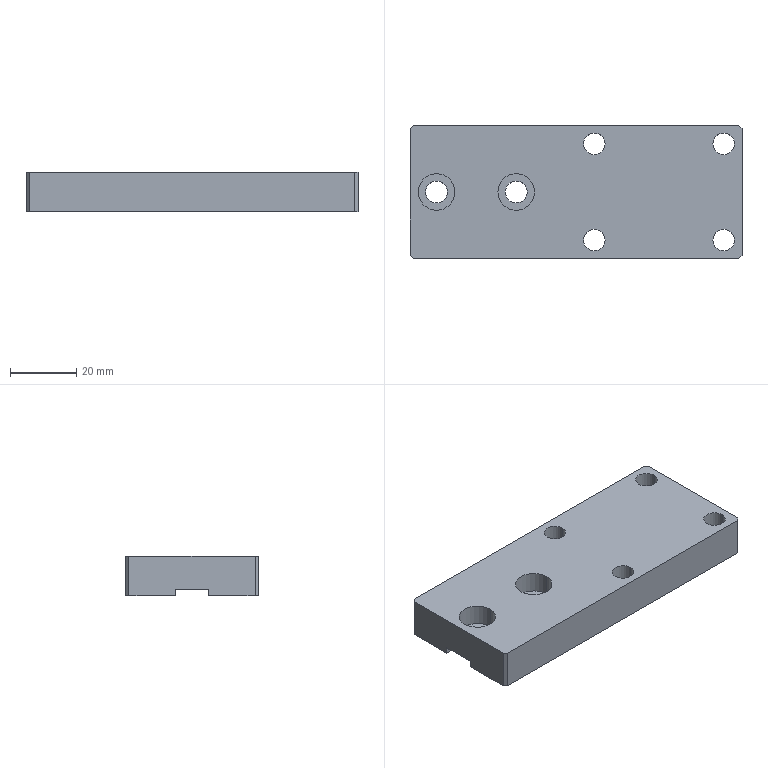Part | STEP file | 11-FG-B04711 | 1 solid | 32 faces | box 100 x 40 x 12 mm | volume 42920 mm3 | cylinder 16 | plane 16 | commonest cylinder face diameters 6.5 x8 6.6 x4 11 x4
STEP:
#1=CARTESIAN_POINT('',(-47.75,34.5,12.));
#2=VERTEX_POINT('',#1);
#3=CARTESIAN_POINT('',(-41.25,34.5,12.));
#4=VERTEX_POINT('',#3);
#5=CARTESIAN_POINT('',(-44.5,34.5,12.));
#6=DIRECTION('',(0.,0.,1.));
#7=DIRECTION('',(1.,0.,0.));
#8=AXIS2_PLACEMENT_3D('',#5,#6,#7);
#9=CIRCLE('',#8,3.25);
#10=EDGE_CURVE('',#2,#4,#9,.T.);
#11=ORIENTED_EDGE('',*,*,#10,.T.);
#12=CARTESIAN_POINT('',(-41.25,34.5,0.));
#13=VERTEX_POINT('',#12);
#14=CARTESIAN_POINT('',(-41.25,34.5,91.));
#15=DIRECTION('',(0.,0.,-1.));
#16=VECTOR('',#15,1000.);
#17=LINE('',#14,#16);
#18=EDGE_CURVE('',#4,#13,#17,.T.);
#19=ORIENTED_EDGE('',*,*,#18,.T.);
#20=CARTESIAN_POINT('',(-47.75,34.5,0.));
#21=VERTEX_POINT('',#20);
#22=CARTESIAN_POINT('',(-44.5,34.5,0.));
#23=DIRECTION('',(0.,0.,-1.));
#24=DIRECTION('',(-1.,0.,0.));
#25=AXIS2_PLACEMENT_3D('',#22,#23,#24);
#26=CIRCLE('',#25,3.25);
#27=EDGE_CURVE('',#13,#21,#26,.T.);
#28=ORIENTED_EDGE('',*,*,#27,.T.);
#29=CARTESIAN_POINT('',(-47.75,34.5,91.));
#30=DIRECTION('',(0.,0.,-1.));
#31=VECTOR('',#30,1000.);
#32=LINE('',#29,#31);
#33=EDGE_CURVE('',#2,#21,#32,.T.);
#34=ORIENTED_EDGE('',*,*,#33,.F.);
#35=EDGE_LOOP('',(#11,#19,#28,#34));
#36=FACE_OUTER_BOUND('',#35,.T.);
#37=CARTESIAN_POINT('',(-44.5,34.5,91.));
#38=DIRECTION('',(0.,0.,-1.));
#39=DIRECTION('',(-1.,0.,0.));
#40=AXIS2_PLACEMENT_3D('',#37,#38,#39);
#41=CYLINDRICAL_SURFACE('',#40,3.25);
#42=ADVANCED_FACE('',(#36),#41,.F.);
#43=CARTESIAN_POINT('',(-8.75,34.5,12.));
#44=VERTEX_POINT('',#43);
#45=CARTESIAN_POINT('',(-2.25,34.5,12.));
#46=VERTEX_POINT('',#45);
#47=CARTESIAN_POINT('',(-5.5,34.5,12.));
#48=DIRECTION('',(0.,0.,1.));
#49=DIRECTION('',(1.,0.,0.));
#50=AXIS2_PLACEMENT_3D('',#47,#48,#49);
#51=CIRCLE('',#50,3.25);
#52=EDGE_CURVE('',#44,#46,#51,.T.);
#53=ORIENTED_EDGE('',*,*,#52,.T.);
#54=CARTESIAN_POINT('',(-2.25,34.5,0.));
#55=VERTEX_POINT('',#54);
#56=CARTESIAN_POINT('',(-2.25,34.5,91.));
#57=DIRECTION('',(0.,0.,-1.));
#58=VECTOR('',#57,1000.);
#59=LINE('',#56,#58);
#60=EDGE_CURVE('',#46,#55,#59,.T.);
#61=ORIENTED_EDGE('',*,*,#60,.T.);
#62=CARTESIAN_POINT('',(-8.75,34.5,0.));
#63=VERTEX_POINT('',#62);
#64=CARTESIAN_POINT('',(-5.5,34.5,0.));
#65=DIRECTION('',(0.,0.,-1.));
#66=DIRECTION('',(-1.,0.,0.));
#67=AXIS2_PLACEMENT_3D('',#64,#65,#66);
#68=CIRCLE('',#67,3.25);
#69=EDGE_CURVE('',#55,#63,#68,.T.);
#70=ORIENTED_EDGE('',*,*,#69,.T.);
#71=CARTESIAN_POINT('',(-8.75,34.5,91.));
#72=DIRECTION('',(0.,0.,-1.));
#73=VECTOR('',#72,1000.);
#74=LINE('',#71,#73);
#75=EDGE_CURVE('',#44,#63,#74,.T.);
#76=ORIENTED_EDGE('',*,*,#75,.F.);
#77=EDGE_LOOP('',(#53,#61,#70,#76));
#78=FACE_OUTER_BOUND('',#77,.T.);
#79=CARTESIAN_POINT('',(-5.5,34.5,91.));
#80=DIRECTION('',(0.,0.,-1.));
#81=DIRECTION('',(-1.,0.,0.));
#82=AXIS2_PLACEMENT_3D('',#79,#80,#81);
#83=CYLINDRICAL_SURFACE('',#82,3.25);
#84=ADVANCED_FACE('',(#78),#83,.F.);
#85=CARTESIAN_POINT('',(-8.75,5.5,12.));
#86=VERTEX_POINT('',#85);
#87=CARTESIAN_POINT('',(-2.25,5.5,12.));
#88=VERTEX_POINT('',#87);
#89=CARTESIAN_POINT('',(-5.5,5.5,12.));
#90=DIRECTION('',(0.,0.,1.));
#91=DIRECTION('',(1.,0.,0.));
#92=AXIS2_PLACEMENT_3D('',#89,#90,#91);
#93=CIRCLE('',#92,3.25);
#94=EDGE_CURVE('',#86,#88,#93,.T.);
#95=ORIENTED_EDGE('',*,*,#94,.T.);
#96=CARTESIAN_POINT('',(-2.25,5.5,0.));
#97=VERTEX_POINT('',#96);
#98=CARTESIAN_POINT('',(-2.25,5.5,91.));
#99=DIRECTION('',(0.,0.,-1.));
#100=VECTOR('',#99,1000.);
#101=LINE('',#98,#100);
#102=EDGE_CURVE('',#88,#97,#101,.T.);
#103=ORIENTED_EDGE('',*,*,#102,.T.);
#104=CARTESIAN_POINT('',(-8.75,5.5,0.));
#105=VERTEX_POINT('',#104);
#106=CARTESIAN_POINT('',(-5.5,5.5,0.));
#107=DIRECTION('',(0.,0.,-1.));
#108=DIRECTION('',(-1.,0.,0.));
#109=AXIS2_PLACEMENT_3D('',#106,#107,#108);
#110=CIRCLE('',#109,3.25);
#111=EDGE_CURVE('',#97,#105,#110,.T.);
#112=ORIENTED_EDGE('',*,*,#111,.T.);
#113=CARTESIAN_POINT('',(-8.75,5.5,91.));
#114=DIRECTION('',(0.,0.,-1.));
#115=VECTOR('',#114,1000.);
#116=LINE('',#113,#115);
#117=EDGE_CURVE('',#86,#105,#116,.T.);
#118=ORIENTED_EDGE('',*,*,#117,.F.);
#119=EDGE_LOOP('',(#95,#103,#112,#118));
#120=FACE_OUTER_BOUND('',#119,.T.);
#121=CARTESIAN_POINT('',(-5.5,5.5,91.));
#122=DIRECTION('',(0.,0.,-1.));
#123=DIRECTION('',(-1.,0.,0.));
#124=AXIS2_PLACEMENT_3D('',#121,#122,#123);
#125=CYLINDRICAL_SURFACE('',#124,3.25);
#126=ADVANCED_FACE('',(#120),#125,.F.);
#127=CARTESIAN_POINT('',(-47.75,5.5,12.));
#128=VERTEX_POINT('',#127);
#129=CARTESIAN_POINT('',(-41.25,5.5,12.));
#130=VERTEX_POINT('',#129);
#131=CARTESIAN_POINT('',(-44.5,5.5,12.));
#132=DIRECTION('',(0.,0.,1.));
#133=DIRECTION('',(1.,0.,0.));
#134=AXIS2_PLACEMENT_3D('',#131,#132,#133);
#135=CIRCLE('',#134,3.25);
#136=EDGE_CURVE('',#128,#130,#135,.T.);
#137=ORIENTED_EDGE('',*,*,#136,.T.);
#138=CARTESIAN_POINT('',(-41.25,5.5,0.));
#139=VERTEX_POINT('',#138);
#140=CARTESIAN_POINT('',(-41.25,5.5,91.));
#141=DIRECTION('',(0.,0.,-1.));
#142=VECTOR('',#141,1000.);
#143=LINE('',#140,#142);
#144=EDGE_CURVE('',#130,#139,#143,.T.);
#145=ORIENTED_EDGE('',*,*,#144,.T.);
#146=CARTESIAN_POINT('',(-47.75,5.5,0.));
#147=VERTEX_POINT('',#146);
#148=CARTESIAN_POINT('',(-44.5,5.5,0.));
#149=DIRECTION('',(0.,0.,-1.));
#150=DIRECTION('',(-1.,0.,0.));
#151=AXIS2_PLACEMENT_3D('',#148,#149,#150);
#152=CIRCLE('',#151,3.25);
#153=EDGE_CURVE('',#139,#147,#152,.T.);
#154=ORIENTED_EDGE('',*,*,#153,.T.);
#155=CARTESIAN_POINT('',(-47.75,5.5,91.));
#156=DIRECTION('',(0.,0.,-1.));
#157=VECTOR('',#156,1000.);
#158=LINE('',#155,#157);
#159=EDGE_CURVE('',#128,#147,#158,.T.);
#160=ORIENTED_EDGE('',*,*,#159,.F.);
#161=EDGE_LOOP('',(#137,#145,#154,#160));
#162=FACE_OUTER_BOUND('',#161,.T.);
#163=CARTESIAN_POINT('',(-44.5,5.5,91.));
#164=DIRECTION('',(0.,0.,-1.));
#165=DIRECTION('',(-1.,0.,0.));
#166=AXIS2_PLACEMENT_3D('',#163,#164,#165);
#167=CYLINDRICAL_SURFACE('',#166,3.25);
#168=ADVANCED_FACE('',(#162),#167,.F.);
#169=CARTESIAN_POINT('',(-97.5,20.,5.6));
#170=VERTEX_POINT('',#169);
#171=CARTESIAN_POINT('',(-86.5,20.,5.6));
#172=VERTEX_POINT('',#171);
#173=CARTESIAN_POINT('',(-92.,20.,5.6));
#174=DIRECTION('',(0.,0.,1.));
#175=DIRECTION('',(1.,0.,0.));
#176=AXIS2_PLACEMENT_3D('',#173,#174,#175);
#177=CIRCLE('',#176,5.5);
#178=EDGE_CURVE('',#170,#172,#177,.T.);
#179=ORIENTED_EDGE('',*,*,#178,.F.);
#180=CARTESIAN_POINT('',(-97.5,20.,12.));
#181=VERTEX_POINT('',#180);
#182=CARTESIAN_POINT('',(-97.5,20.,12.));
#183=DIRECTION('',(0.,0.,1.));
#184=VECTOR('',#183,1000.);
#185=LINE('',#182,#184);
#186=EDGE_CURVE('',#170,#181,#185,.T.);
#187=ORIENTED_EDGE('',*,*,#186,.T.);
#188=CARTESIAN_POINT('',(-86.5,20.,12.));
#189=VERTEX_POINT('',#188);
#190=CARTESIAN_POINT('',(-92.,20.,12.));
#191=DIRECTION('',(0.,0.,1.));
#192=DIRECTION('',(1.,0.,0.));
#193=AXIS2_PLACEMENT_3D('',#190,#191,#192);
#194=CIRCLE('',#193,5.5);
#195=EDGE_CURVE('',#181,#189,#194,.T.);
#196=ORIENTED_EDGE('',*,*,#195,.T.);
#197=CARTESIAN_POINT('',(-86.5,20.,12.));
#198=DIRECTION('',(0.,0.,1.));
#199=VECTOR('',#198,1000.);
#200=LINE('',#197,#199);
#201=EDGE_CURVE('',#172,#189,#200,.T.);
#202=ORIENTED_EDGE('',*,*,#201,.F.);
#203=EDGE_LOOP('',(#179,#187,#196,#202));
#204=FACE_OUTER_BOUND('',#203,.T.);
#205=CARTESIAN_POINT('',(-92.,20.,12.));
#206=DIRECTION('',(0.,0.,1.));
#207=DIRECTION('',(1.,0.,0.));
#208=AXIS2_PLACEMENT_3D('',#205,#206,#207);
#209=CYLINDRICAL_SURFACE('',#208,5.5);
#210=ADVANCED_FACE('',(#204),#209,.F.);
#211=CARTESIAN_POINT('',(-95.3,20.,2.));
#212=VERTEX_POINT('',#211);
#213=CARTESIAN_POINT('',(-88.7,20.,2.));
#214=VERTEX_POINT('',#213);
#215=CARTESIAN_POINT('',(-92.,20.,2.));
#216=DIRECTION('',(0.,0.,1.));
#217=DIRECTION('',(1.,0.,0.));
#218=AXIS2_PLACEMENT_3D('',#215,#216,#217);
#219=CIRCLE('',#218,3.3);
#220=EDGE_CURVE('',#212,#214,#219,.T.);
#221=ORIENTED_EDGE('',*,*,#220,.F.);
#222=CARTESIAN_POINT('',(-95.3,20.,5.6));
#223=VERTEX_POINT('',#222);
#224=CARTESIAN_POINT('',(-95.3,20.,12.));
#225=DIRECTION('',(0.,0.,1.));
#226=VECTOR('',#225,1000.);
#227=LINE('',#224,#226);
#228=EDGE_CURVE('',#212,#223,#227,.T.);
#229=ORIENTED_EDGE('',*,*,#228,.T.);
#230=CARTESIAN_POINT('',(-88.7,20.,5.6));
#231=VERTEX_POINT('',#230);
#232=CARTESIAN_POINT('',(-92.,20.,5.6));
#233=DIRECTION('',(0.,0.,1.));
#234=DIRECTION('',(1.,0.,0.));
#235=AXIS2_PLACEMENT_3D('',#232,#233,#234);
#236=CIRCLE('',#235,3.3);
#237=EDGE_CURVE('',#223,#231,#236,.T.);
#238=ORIENTED_EDGE('',*,*,#237,.T.);
#239=CARTESIAN_POINT('',(-88.7,20.,12.));
#240=DIRECTION('',(0.,0.,1.));
#241=VECTOR('',#240,1000.);
#242=LINE('',#239,#241);
#243=EDGE_CURVE('',#214,#231,#242,.T.);
#244=ORIENTED_EDGE('',*,*,#243,.F.);
#245=EDGE_LOOP('',(#221,#229,#238,#244));
#246=FACE_OUTER_BOUND('',#245,.T.);
#247=CARTESIAN_POINT('',(-92.,20.,12.));
#248=DIRECTION('',(0.,0.,1.));
#249=DIRECTION('',(1.,0.,0.));
#250=AXIS2_PLACEMENT_3D('',#247,#248,#249);
#251=CYLINDRICAL_SURFACE('',#250,3.3);
#252=ADVANCED_FACE('',(#246),#251,.F.);
#253=CARTESIAN_POINT('',(-73.5,20.,5.6));
#254=VERTEX_POINT('',#253);
#255=CARTESIAN_POINT('',(-62.5,20.,5.6));
#256=VERTEX_POINT('',#255);
#257=CARTESIAN_POINT('',(-68.,20.,5.6));
#258=DIRECTION('',(0.,0.,1.));
#259=DIRECTION('',(1.,0.,0.));
#260=AXIS2_PLACEMENT_3D('',#257,#258,#259);
#261=CIRCLE('',#260,5.5);
#262=EDGE_CURVE('',#254,#256,#261,.T.);
#263=ORIENTED_EDGE('',*,*,#262,.F.);
#264=CARTESIAN_POINT('',(-73.5,20.,12.));
#265=VERTEX_POINT('',#264);
#266=CARTESIAN_POINT('',(-73.5,20.,12.));
#267=DIRECTION('',(0.,0.,1.));
#268=VECTOR('',#267,1000.);
#269=LINE('',#266,#268);
#270=EDGE_CURVE('',#254,#265,#269,.T.);
#271=ORIENTED_EDGE('',*,*,#270,.T.);
#272=CARTESIAN_POINT('',(-62.5,20.,12.));
#273=VERTEX_POINT('',#272);
#274=CARTESIAN_POINT('',(-68.,20.,12.));
#275=DIRECTION('',(0.,0.,1.));
#276=DIRECTION('',(1.,0.,0.));
#277=AXIS2_PLACEMENT_3D('',#274,#275,#276);
#278=CIRCLE('',#277,5.5);
#279=EDGE_CURVE('',#265,#273,#278,.T.);
#280=ORIENTED_EDGE('',*,*,#279,.T.);
#281=CARTESIAN_POINT('',(-62.5,20.,12.));
#282=DIRECTION('',(0.,0.,1.));
#283=VECTOR('',#282,1000.);
#284=LINE('',#281,#283);
#285=EDGE_CURVE('',#256,#273,#284,.T.);
#286=ORIENTED_EDGE('',*,*,#285,.F.);
#287=EDGE_LOOP('',(#263,#271,#280,#286));
#288=FACE_OUTER_BOUND('',#287,.T.);
#289=CARTESIAN_POINT('',(-68.,20.,12.));
#290=DIRECTION('',(0.,0.,1.));
#291=DIRECTION('',(1.,0.,0.));
#292=AXIS2_PLACEMENT_3D('',#289,#290,#291);
#293=CYLINDRICAL_SURFACE('',#292,5.5);
#294=ADVANCED_FACE('',(#288),#293,.F.);
#295=CARTESIAN_POINT('',(-71.3,20.,2.));
#296=VERTEX_POINT('',#295);
#297=CARTESIAN_POINT('',(-64.7,20.,2.));
#298=VERTEX_POINT('',#297);
#299=CARTESIAN_POINT('',(-68.,20.,2.));
#300=DIRECTION('',(0.,0.,1.));
#301=DIRECTION('',(1.,0.,0.));
#302=AXIS2_PLACEMENT_3D('',#299,#300,#301);
#303=CIRCLE('',#302,3.3);
#304=EDGE_CURVE('',#296,#298,#303,.T.);
#305=ORIENTED_EDGE('',*,*,#304,.F.);
#306=CARTESIAN_POINT('',(-71.3,20.,5.6));
#307=VERTEX_POINT('',#306);
#308=CARTESIAN_POINT('',(-71.3,20.,12.));
#309=DIRECTION('',(0.,0.,1.));
#310=VECTOR('',#309,1000.);
#311=LINE('',#308,#310);
#312=EDGE_CURVE('',#296,#307,#311,.T.);
#313=ORIENTED_EDGE('',*,*,#312,.T.);
#314=CARTESIAN_POINT('',(-64.7,20.,5.6));
#315=VERTEX_POINT('',#314);
#316=CARTESIAN_POINT('',(-68.,20.,5.6));
#317=DIRECTION('',(0.,0.,1.));
#318=DIRECTION('',(1.,0.,0.));
#319=AXIS2_PLACEMENT_3D('',#316,#317,#318);
#320=CIRCLE('',#319,3.3);
#321=EDGE_CURVE('',#307,#315,#320,.T.);
#322=ORIENTED_EDGE('',*,*,#321,.T.);
#323=CARTESIAN_POINT('',(-64.7,20.,12.));
#324=DIRECTION('',(0.,0.,1.));
#325=VECTOR('',#324,1000.);
#326=LINE('',#323,#325);
#327=EDGE_CURVE('',#298,#315,#326,.T.);
#328=ORIENTED_EDGE('',*,*,#327,.F.);
#329=EDGE_LOOP('',(#305,#313,#322,#328));
#330=FACE_OUTER_BOUND('',#329,.T.);
#331=CARTESIAN_POINT('',(-68.,20.,12.));
#332=DIRECTION('',(0.,0.,1.));
#333=DIRECTION('',(1.,0.,0.));
#334=AXIS2_PLACEMENT_3D('',#331,#332,#333);
#335=CYLINDRICAL_SURFACE('',#334,3.3);
#336=ADVANCED_FACE('',(#330),#335,.F.);
#337=CARTESIAN_POINT('',(-44.5,34.5,0.));
#338=DIRECTION('',(0.,0.,-1.));
#339=DIRECTION('',(-1.,0.,0.));
#340=AXIS2_PLACEMENT_3D('',#337,#338,#339);
#341=CIRCLE('',#340,3.25);
#342=EDGE_CURVE('',#21,#13,#341,.T.);
#343=ORIENTED_EDGE('',*,*,#342,.F.);
#344=ORIENTED_EDGE('',*,*,#27,.F.);
#345=EDGE_LOOP('',(#343,#344));
#346=FACE_BOUND('',#345,.T.);
#347=CARTESIAN_POINT('',(-5.5,34.5,0.));
#348=DIRECTION('',(0.,0.,-1.));
#349=DIRECTION('',(-1.,0.,0.));
#350=AXIS2_PLACEMENT_3D('',#347,#348,#349);
#351=CIRCLE('',#350,3.25);
#352=EDGE_CURVE('',#63,#55,#351,.T.);
#353=ORIENTED_EDGE('',*,*,#352,.F.);
#354=ORIENTED_EDGE('',*,*,#69,.F.);
#355=EDGE_LOOP('',(#353,#354));
#356=FACE_BOUND('',#355,.T.);
#357=CARTESIAN_POINT('',(0.,25.,0.));
#358=VERTEX_POINT('',#357);
#359=CARTESIAN_POINT('',(0.,39.,0.));
#360=VERTEX_POINT('',#359);
#361=CARTESIAN_POINT('',(0.,40.,0.));
#362=DIRECTION('',(0.,1.,0.));
#363=VECTOR('',#362,1000.);
#364=LINE('',#361,#363);
#365=EDGE_CURVE('',#358,#360,#364,.T.);
#366=ORIENTED_EDGE('',*,*,#365,.F.);
#367=CARTESIAN_POINT('',(-100.,25.,0.));
#368=VERTEX_POINT('',#367);
#369=CARTESIAN_POINT('',(-100.,25.,0.));
#370=DIRECTION('',(-1.,0.,0.));
#371=VECTOR('',#370,1000.);
#372=LINE('',#369,#371);
#373=EDGE_CURVE('',#358,#368,#372,.T.);
#374=ORIENTED_EDGE('',*,*,#373,.T.);
#375=CARTESIAN_POINT('',(-100.,39.,0.));
#376=VERTEX_POINT('',#375);
#377=CARTESIAN_POINT('',(-100.,40.,0.));
#378=DIRECTION('',(0.,-1.,0.));
#379=VECTOR('',#378,1000.);
#380=LINE('',#377,#379);
#381=EDGE_CURVE('',#376,#368,#380,.T.);
#382=ORIENTED_EDGE('',*,*,#381,.F.);
#383=CARTESIAN_POINT('',(-99.,40.,0.));
#384=VERTEX_POINT('',#383);
#385=CARTESIAN_POINT('',(-100.,39.,0.));
#386=DIRECTION('',(0.7071,0.7071,0.));
#387=VECTOR('',#386,1000.);
#388=LINE('',#385,#387);
#389=EDGE_CURVE('',#376,#384,#388,.T.);
#390=ORIENTED_EDGE('',*,*,#389,.T.);
#391=CARTESIAN_POINT('',(-1.,40.,0.));
#392=VERTEX_POINT('',#391);
#393=CARTESIAN_POINT('',(-100.,40.,0.));
#394=DIRECTION('',(-1.,0.,0.));
#395=VECTOR('',#394,1000.);
#396=LINE('',#393,#395);
#397=EDGE_CURVE('',#392,#384,#396,.T.);
#398=ORIENTED_EDGE('',*,*,#397,.F.);
#399=CARTESIAN_POINT('',(-1.,40.,0.));
#400=DIRECTION('',(0.7071,-0.7071,0.));
#401=VECTOR('',#400,1000.);
#402=LINE('',#399,#401);
#403=EDGE_CURVE('',#392,#360,#402,.T.);
#404=ORIENTED_EDGE('',*,*,#403,.T.);
#405=EDGE_LOOP('',(#366,#374,#382,#390,#398,#404));
#406=FACE_OUTER_BOUND('',#405,.T.);
#407=CARTESIAN_POINT('',(-100.,0.,0.));
#408=DIRECTION('',(0.,0.,1.));
#409=DIRECTION('',(1.,0.,0.));
#410=AXIS2_PLACEMENT_3D('',#407,#408,#409);
#411=PLANE('',#410);
#412=ADVANCED_FACE('',(#346,#356,#406),#411,.F.);
#413=ORIENTED_EDGE('',*,*,#381,.T.);
#414=CARTESIAN_POINT('',(-100.,25.,2.));
#415=VERTEX_POINT('',#414);
#416=CARTESIAN_POINT('',(-100.,25.,0.));
#417=DIRECTION('',(0.,0.,-1.));
#418=VECTOR('',#417,1000.);
#419=LINE('',#416,#418);
#420=EDGE_CURVE('',#415,#368,#419,.T.);
#421=ORIENTED_EDGE('',*,*,#420,.F.);
#422=CARTESIAN_POINT('',(-100.,15.,2.));
#423=VERTEX_POINT('',#422);
#424=CARTESIAN_POINT('',(-100.,15.,2.));
#425=DIRECTION('',(0.,1.,0.));
#426=VECTOR('',#425,1000.);
#427=LINE('',#424,#426);
#428=EDGE_CURVE('',#423,#415,#427,.T.);
#429=ORIENTED_EDGE('',*,*,#428,.F.);
#430=CARTESIAN_POINT('',(-100.,15.,0.));
#431=VERTEX_POINT('',#430);
#432=CARTESIAN_POINT('',(-100.,15.,0.));
#433=DIRECTION('',(0.,0.,1.));
#434=VECTOR('',#433,1000.);
#435=LINE('',#432,#434);
#436=EDGE_CURVE('',#431,#423,#435,.T.);
#437=ORIENTED_EDGE('',*,*,#436,.F.);
#438=CARTESIAN_POINT('',(-100.,1.,0.));
#439=VERTEX_POINT('',#438);
#440=CARTESIAN_POINT('',(-100.,40.,0.));
#441=DIRECTION('',(0.,-1.,0.));
#442=VECTOR('',#441,1000.);
#443=LINE('',#440,#442);
#444=EDGE_CURVE('',#431,#439,#443,.T.);
#445=ORIENTED_EDGE('',*,*,#444,.T.);
#446=CARTESIAN_POINT('',(-100.,1.,12.));
#447=VERTEX_POINT('',#446);
#448=CARTESIAN_POINT('',(-100.,1.,12.));
#449=DIRECTION('',(0.,0.,1.));
#450=VECTOR('',#449,1000.);
#451=LINE('',#448,#450);
#452=EDGE_CURVE('',#439,#447,#451,.T.);
#453=ORIENTED_EDGE('',*,*,#452,.T.);
#454=CARTESIAN_POINT('',(-100.,39.,12.));
#455=VERTEX_POINT('',#454);
#456=CARTESIAN_POINT('',(-100.,40.,12.));
#457=DIRECTION('',(0.,-1.,0.));
#458=VECTOR('',#457,1000.);
#459=LINE('',#456,#458);
#460=EDGE_CURVE('',#455,#447,#459,.T.);
#461=ORIENTED_EDGE('',*,*,#460,.F.);
#462=CARTESIAN_POINT('',(-100.,39.,12.));
#463=DIRECTION('',(0.,0.,-1.));
#464=VECTOR('',#463,1000.);
#465=LINE('',#462,#464);
#466=EDGE_CURVE('',#455,#376,#465,.T.);
#467=ORIENTED_EDGE('',*,*,#466,.T.);
#468=EDGE_LOOP('',(#413,#421,#429,#437,#445,#453,#461,#467));
#469=FACE_OUTER_BOUND('',#468,.T.);
#470=CARTESIAN_POINT('',(-100.,40.,12.));
#471=DIRECTION('',(1.,0.,0.));
#472=DIRECTION('',(0.,0.,-1.));
#473=AXIS2_PLACEMENT_3D('',#470,#471,#472);
#474=PLANE('',#473);
#475=ADVANCED_FACE('',(#469),#474,.F.);
#476=CARTESIAN_POINT('',(-99.,0.,12.));
#477=VERTEX_POINT('',#476);
#478=CARTESIAN_POINT('',(-1.,0.,12.));
#479=VERTEX_POINT('',#478);
#480=CARTESIAN_POINT('',(-100.,0.,12.));
#481=DIRECTION('',(1.,0.,0.));
#482=VECTOR('',#481,1000.);
#483=LINE('',#480,#482);
#484=EDGE_CURVE('',#477,#479,#483,.T.);
#485=ORIENTED_EDGE('',*,*,#484,.F.);
#486=CARTESIAN_POINT('',(-99.,0.,0.));
#487=VERTEX_POINT('',#486);
#488=CARTESIAN_POINT('',(-99.,0.,12.));
#489=DIRECTION('',(0.,0.,-1.));
#490=VECTOR('',#489,1000.);
#491=LINE('',#488,#490);
#492=EDGE_CURVE('',#477,#487,#491,.T.);
#493=ORIENTED_EDGE('',*,*,#492,.T.);
#494=CARTESIAN_POINT('',(-1.,0.,0.));
#495=VERTEX_POINT('',#494);
#496=CARTESIAN_POINT('',(-100.,0.,0.));
#497=DIRECTION('',(1.,0.,0.));
#498=VECTOR('',#497,1000.);
#499=LINE('',#496,#498);
#500=EDGE_CURVE('',#487,#495,#499,.T.);
#501=ORIENTED_EDGE('',*,*,#500,.T.);
#502=CARTESIAN_POINT('',(-1.,0.,12.));
#503=DIRECTION('',(0.,0.,1.));
#504=VECTOR('',#503,1000.);
#505=LINE('',#502,#504);
#506=EDGE_CURVE('',#495,#479,#505,.T.);
#507=ORIENTED_EDGE('',*,*,#506,.T.);
#508=EDGE_LOOP('',(#485,#493,#501,#507));
#509=FACE_OUTER_BOUND('',#508,.T.);
#510=CARTESIAN_POINT('',(-100.,0.,12.));
#511=DIRECTION('',(0.,1.,0.));
#512=DIRECTION('',(0.,0.,1.));
#513=AXIS2_PLACEMENT_3D('',#510,#511,#512);
#514=PLANE('',#513);
#515=ADVANCED_FACE('',(#509),#514,.F.);
#516=CARTESIAN_POINT('',(0.,15.,2.));
#517=VERTEX_POINT('',#516);
#518=CARTESIAN_POINT('',(0.,25.,2.));
#519=VERTEX_POINT('',#518);
#520=CARTESIAN_POINT('',(0.,40.,2.));
#521=DIRECTION('',(0.,1.,0.));
#522=VECTOR('',#521,1000.);
#523=LINE('',#520,#522);
#524=EDGE_CURVE('',#517,#519,#523,.T.);
#525=ORIENTED_EDGE('',*,*,#524,.T.);
#526=CARTESIAN_POINT('',(0.,25.,12.));
#527=DIRECTION('',(0.,0.,-1.));
#528=VECTOR('',#527,1000.);
#529=LINE('',#526,#528);
#530=EDGE_CURVE('',#519,#358,#529,.T.);
#531=ORIENTED_EDGE('',*,*,#530,.T.);
#532=ORIENTED_EDGE('',*,*,#365,.T.);
#533=CARTESIAN_POINT('',(0.,39.,12.));
#534=VERTEX_POINT('',#533);
#535=CARTESIAN_POINT('',(0.,39.,12.));
#536=DIRECTION('',(0.,0.,1.));
#537=VECTOR('',#536,1000.);
#538=LINE('',#535,#537);
#539=EDGE_CURVE('',#360,#534,#538,.T.);
#540=ORIENTED_EDGE('',*,*,#539,.T.);
#541=CARTESIAN_POINT('',(0.,1.,12.));
#542=VERTEX_POINT('',#541);
#543=CARTESIAN_POINT('',(0.,40.,12.));
#544=DIRECTION('',(0.,1.,0.));
#545=VECTOR('',#544,1000.);
#546=LINE('',#543,#545);
#547=EDGE_CURVE('',#542,#534,#546,.T.);
#548=ORIENTED_EDGE('',*,*,#547,.F.);
#549=CARTESIAN_POINT('',(0.,1.,0.));
#550=VERTEX_POINT('',#549);
#551=CARTESIAN_POINT('',(0.,1.,12.));
#552=DIRECTION('',(0.,0.,-1.));
#553=VECTOR('',#552,1000.);
#554=LINE('',#551,#553);
#555=EDGE_CURVE('',#542,#550,#554,.T.);
#556=ORIENTED_EDGE('',*,*,#555,.T.);
#557=CARTESIAN_POINT('',(0.,15.,0.));
#558=VERTEX_POINT('',#557);
#559=CARTESIAN_POINT('',(0.,40.,0.));
#560=DIRECTION('',(0.,1.,0.));
#561=VECTOR('',#560,1000.);
#562=LINE('',#559,#561);
#563=EDGE_CURVE('',#550,#558,#562,.T.);
#564=ORIENTED_EDGE('',*,*,#563,.T.);
#565=CARTESIAN_POINT('',(0.,15.,12.));
#566=DIRECTION('',(0.,0.,1.));
#567=VECTOR('',#566,1000.);
#568=LINE('',#565,#567);
#569=EDGE_CURVE('',#558,#517,#568,.T.);
#570=ORIENTED_EDGE('',*,*,#569,.T.);
#571=EDGE_LOOP('',(#525,#531,#532,#540,#548,#556,#564,#570));
#572=FACE_OUTER_BOUND('',#571,.T.);
#573=CARTESIAN_POINT('',(0.,40.,12.));
#574=DIRECTION('',(-1.,0.,0.));
#575=DIRECTION('',(0.,-1.,0.));
#576=AXIS2_PLACEMENT_3D('',#573,#574,#575);
#577=PLANE('',#576);
#578=ADVANCED_FACE('',(#572),#577,.F.);
#579=CARTESIAN_POINT('',(-1.,40.,12.));
#580=VERTEX_POINT('',#579);
#581=CARTESIAN_POINT('',(-99.,40.,12.));
#582=VERTEX_POINT('',#581);
#583=CARTESIAN_POINT('',(-100.,40.,12.));
#584=DIRECTION('',(-1.,0.,0.));
#585=VECTOR('',#584,1000.);
#586=LINE('',#583,#585);
#587=EDGE_CURVE('',#580,#582,#586,.T.);
#588=ORIENTED_EDGE('',*,*,#587,.F.);
#589=CARTESIAN_POINT('',(-1.,40.,12.));
#590=DIRECTION('',(0.,0.,-1.));
#591=VECTOR('',#590,1000.);
#592=LINE('',#589,#591);
#593=EDGE_CURVE('',#580,#392,#592,.T.);
#594=ORIENTED_EDGE('',*,*,#593,.T.);
#595=ORIENTED_EDGE('',*,*,#397,.T.);
#596=CARTESIAN_POINT('',(-99.,40.,12.));
#597=DIRECTION('',(0.,0.,1.));
#598=VECTOR('',#597,1000.);
#599=LINE('',#596,#598);
#600=EDGE_CURVE('',#384,#582,#599,.T.);
#601=ORIENTED_EDGE('',*,*,#600,.T.);
#602=EDGE_LOOP('',(#588,#594,#595,#601));
#603=FACE_OUTER_BOUND('',#602,.T.);
#604=CARTESIAN_POINT('',(-100.,40.,12.));
#605=DIRECTION('',(0.,-1.,0.));
#606=DIRECTION('',(0.,0.,-1.));
#607=AXIS2_PLACEMENT_3D('',#604,#605,#606);
#608=PLANE('',#607);
#609=ADVANCED_FACE('',(#603),#608,.F.);
#610=ORIENTED_EDGE('',*,*,#94,.F.);
#611=CARTESIAN_POINT('',(-5.5,5.5,12.));
#612=DIRECTION('',(0.,0.,1.));
#613=DIRECTION('',(1.,0.,0.));
#614=AXIS2_PLACEMENT_3D('',#611,#612,#613);
#615=CIRCLE('',#614,3.25);
#616=EDGE_CURVE('',#88,#86,#615,.T.);
#617=ORIENTED_EDGE('',*,*,#616,.F.);
#618=EDGE_LOOP('',(#610,#617));
#619=FACE_BOUND('',#618,.T.);
#620=ORIENTED_EDGE('',*,*,#10,.F.);
#621=CARTESIAN_POINT('',(-44.5,34.5,12.));
#622=DIRECTION('',(0.,0.,1.));
#623=DIRECTION('',(1.,0.,0.));
#624=AXIS2_PLACEMENT_3D('',#621,#622,#623);
#625=CIRCLE('',#624,3.25);
#626=EDGE_CURVE('',#4,#2,#625,.T.);
#627=ORIENTED_EDGE('',*,*,#626,.F.);
#628=EDGE_LOOP('',(#620,#627));
#629=FACE_BOUND('',#628,.T.);
#630=ORIENTED_EDGE('',*,*,#52,.F.);
#631=CARTESIAN_POINT('',(-5.5,34.5,12.));
#632=DIRECTION('',(0.,0.,1.));
#633=DIRECTION('',(1.,0.,0.));
#634=AXIS2_PLACEMENT_3D('',#631,#632,#633);
#635=CIRCLE('',#634,3.25);
#636=EDGE_CURVE('',#46,#44,#635,.T.);
#637=ORIENTED_EDGE('',*,*,#636,.F.);
#638=EDGE_LOOP('',(#630,#637));
#639=FACE_BOUND('',#638,.T.);
#640=ORIENTED_EDGE('',*,*,#136,.F.);
#641=CARTESIAN_POINT('',(-44.5,5.5,12.));
#642=DIRECTION('',(0.,0.,1.));
#643=DIRECTION('',(1.,0.,0.));
#644=AXIS2_PLACEMENT_3D('',#641,#642,#643);
#645=CIRCLE('',#644,3.25);
#646=EDGE_CURVE('',#130,#128,#645,.T.);
#647=ORIENTED_EDGE('',*,*,#646,.F.);
#648=EDGE_LOOP('',(#640,#647));
#649=FACE_BOUND('',#648,.T.);
#650=CARTESIAN_POINT('',(-92.,20.,12.));
#651=DIRECTION('',(0.,0.,1.));
#652=DIRECTION('',(1.,0.,0.));
#653=AXIS2_PLACEMENT_3D('',#650,#651,#652);
#654=CIRCLE('',#653,5.5);
#655=EDGE_CURVE('',#189,#181,#654,.T.);
#656=ORIENTED_EDGE('',*,*,#655,.F.);
#657=ORIENTED_EDGE('',*,*,#195,.F.);
#658=EDGE_LOOP('',(#656,#657));
#659=FACE_BOUND('',#658,.T.);
#660=CARTESIAN_POINT('',(-68.,20.,12.));
#661=DIRECTION('',(0.,0.,1.));
#662=DIRECTION('',(1.,0.,0.));
#663=AXIS2_PLACEMENT_3D('',#660,#661,#662);
#664=CIRCLE('',#663,5.5);
#665=EDGE_CURVE('',#273,#265,#664,.T.);
#666=ORIENTED_EDGE('',*,*,#665,.F.);
#667=ORIENTED_EDGE('',*,*,#279,.F.);
#668=EDGE_LOOP('',(#666,#667));
#669=FACE_BOUND('',#668,.T.);
#670=ORIENTED_EDGE('',*,*,#460,.T.);
#671=CARTESIAN_POINT('',(-99.5,0.5,12.));
#672=DIRECTION('',(0.7071,-0.7071,0.));
#673=VECTOR('',#672,1000.);
#674=LINE('',#671,#673);
#675=EDGE_CURVE('',#447,#477,#674,.T.);
#676=ORIENTED_EDGE('',*,*,#675,.T.);
#677=ORIENTED_EDGE('',*,*,#484,.T.);
#678=CARTESIAN_POINT('',(-50.5,-49.5,12.));
#679=DIRECTION('',(0.7071,0.7071,0.));
#680=VECTOR('',#679,1000.);
#681=LINE('',#678,#680);
#682=EDGE_CURVE('',#479,#542,#681,.T.);
#683=ORIENTED_EDGE('',*,*,#682,.T.);
#684=ORIENTED_EDGE('',*,*,#547,.T.);
#685=CARTESIAN_POINT('',(-30.5,69.5,12.));
#686=DIRECTION('',(-0.7071,0.7071,0.));
#687=VECTOR('',#686,1000.);
#688=LINE('',#685,#687);
#689=EDGE_CURVE('',#534,#580,#688,.T.);
#690=ORIENTED_EDGE('',*,*,#689,.T.);
#691=ORIENTED_EDGE('',*,*,#587,.T.);
#692=CARTESIAN_POINT('',(-119.5,19.5,12.));
#693=DIRECTION('',(-0.7071,-0.7071,0.));
#694=VECTOR('',#693,1000.);
#695=LINE('',#692,#694);
#696=EDGE_CURVE('',#582,#455,#695,.T.);
#697=ORIENTED_EDGE('',*,*,#696,.T.);
#698=EDGE_LOOP('',(#670,#676,#677,#683,#684,#690,#691,#697));
#699=FACE_OUTER_BOUND('',#698,.T.);
#700=CARTESIAN_POINT('',(-100.,0.,12.));
#701=DIRECTION('',(0.,0.,1.));
#702=DIRECTION('',(1.,0.,0.));
#703=AXIS2_PLACEMENT_3D('',#700,#701,#702);
#704=PLANE('',#703);
#705=ADVANCED_FACE('',(#619,#629,#639,#649,#659,#669,#699),#704,.T.);
#706=CARTESIAN_POINT('',(-5.5,5.5,0.));
#707=DIRECTION('',(0.,0.,-1.));
#708=DIRECTION('',(-1.,0.,0.));
#709=AXIS2_PLACEMENT_3D('',#706,#707,#708);
#710=CIRCLE('',#709,3.25);
#711=EDGE_CURVE('',#105,#97,#710,.T.);
#712=ORIENTED_EDGE('',*,*,#711,.F.);
#713=ORIENTED_EDGE('',*,*,#111,.F.);
#714=EDGE_LOOP('',(#712,#713));
#715=FACE_BOUND('',#714,.T.);
#716=CARTESIAN_POINT('',(-44.5,5.5,0.));
#717=DIRECTION('',(0.,0.,-1.));
#718=DIRECTION('',(-1.,0.,0.));
#719=AXIS2_PLACEMENT_3D('',#716,#717,#718);
#720=CIRCLE('',#719,3.25);
#721=EDGE_CURVE('',#147,#139,#720,.T.);
#722=ORIENTED_EDGE('',*,*,#721,.F.);
#723=ORIENTED_EDGE('',*,*,#153,.F.);
#724=EDGE_LOOP('',(#722,#723));
#725=FACE_BOUND('',#724,.T.);
#726=ORIENTED_EDGE('',*,*,#444,.F.);
#727=CARTESIAN_POINT('',(-100.,15.,0.));
#728=DIRECTION('',(1.,0.,0.));
#729=VECTOR('',#728,1000.);
#730=LINE('',#727,#729);
#731=EDGE_CURVE('',#431,#558,#730,.T.);
#732=ORIENTED_EDGE('',*,*,#731,.T.);
#733=ORIENTED_EDGE('',*,*,#563,.F.);
#734=CARTESIAN_POINT('',(0.,1.,0.));
#735=DIRECTION('',(-0.7071,-0.7071,0.));
#736=VECTOR('',#735,1000.);
#737=LINE('',#734,#736);
#738=EDGE_CURVE('',#550,#495,#737,.T.);
#739=ORIENTED_EDGE('',*,*,#738,.T.);
#740=ORIENTED_EDGE('',*,*,#500,.F.);
#741=CARTESIAN_POINT('',(-99.,0.,0.));
#742=DIRECTION('',(-0.7071,0.7071,0.));
#743=VECTOR('',#742,1000.);
#744=LINE('',#741,#743);
#745=EDGE_CURVE('',#487,#439,#744,.T.);
#746=ORIENTED_EDGE('',*,*,#745,.T.);
#747=EDGE_LOOP('',(#726,#732,#733,#739,#740,#746));
#748=FACE_OUTER_BOUND('',#747,.T.);
#749=CARTESIAN_POINT('',(-100.,0.,0.));
#750=DIRECTION('',(0.,0.,1.));
#751=DIRECTION('',(1.,0.,0.));
#752=AXIS2_PLACEMENT_3D('',#749,#750,#751);
#753=PLANE('',#752);
#754=ADVANCED_FACE('',(#715,#725,#748),#753,.F.);
#755=ORIENTED_EDGE('',*,*,#675,.F.);
#756=ORIENTED_EDGE('',*,*,#452,.F.);
#757=ORIENTED_EDGE('',*,*,#745,.F.);
#758=ORIENTED_EDGE('',*,*,#492,.F.);
#759=EDGE_LOOP('',(#755,#756,#757,#758));
#760=FACE_OUTER_BOUND('',#759,.T.);
#761=CARTESIAN_POINT('',(-99.,0.,12.));
#762=DIRECTION('',(0.7071,0.7071,0.));
#763=DIRECTION('',(0.,0.,-1.));
#764=AXIS2_PLACEMENT_3D('',#761,#762,#763);
#765=PLANE('',#764);
#766=ADVANCED_FACE('',(#760),#765,.F.);
#767=ORIENTED_EDGE('',*,*,#682,.F.);
#768=ORIENTED_EDGE('',*,*,#506,.F.);
#769=ORIENTED_EDGE('',*,*,#738,.F.);
#770=ORIENTED_EDGE('',*,*,#555,.F.);
#771=EDGE_LOOP('',(#767,#768,#769,#770));
#772=FACE_OUTER_BOUND('',#771,.T.);
#773=CARTESIAN_POINT('',(0.,1.,12.));
#774=DIRECTION('',(-0.7071,0.7071,0.));
#775=DIRECTION('',(0.,0.,-1.));
#776=AXIS2_PLACEMENT_3D('',#773,#774,#775);
#777=PLANE('',#776);
#778=ADVANCED_FACE('',(#772),#777,.F.);
#779=ORIENTED_EDGE('',*,*,#689,.F.);
#780=ORIENTED_EDGE('',*,*,#539,.F.);
#781=ORIENTED_EDGE('',*,*,#403,.F.);
#782=ORIENTED_EDGE('',*,*,#593,.F.);
#783=EDGE_LOOP('',(#779,#780,#781,#782));
#784=FACE_OUTER_BOUND('',#783,.T.);
#785=CARTESIAN_POINT('',(-1.,40.,12.));
#786=DIRECTION('',(-0.7071,-0.7071,0.));
#787=DIRECTION('',(0.,0.,-1.));
#788=AXIS2_PLACEMENT_3D('',#785,#786,#787);
#789=PLANE('',#788);
#790=ADVANCED_FACE('',(#784),#789,.F.);
#791=ORIENTED_EDGE('',*,*,#696,.F.);
#792=ORIENTED_EDGE('',*,*,#600,.F.);
#793=ORIENTED_EDGE('',*,*,#389,.F.);
#794=ORIENTED_EDGE('',*,*,#466,.F.);
#795=EDGE_LOOP('',(#791,#792,#793,#794));
#796=FACE_OUTER_BOUND('',#795,.T.);
#797=CARTESIAN_POINT('',(-100.,39.,12.));
#798=DIRECTION('',(0.7071,-0.7071,0.));
#799=DIRECTION('',(0.,0.,-1.));
#800=AXIS2_PLACEMENT_3D('',#797,#798,#799);
#801=PLANE('',#800);
#802=ADVANCED_FACE('',(#796),#801,.F.);
#803=CARTESIAN_POINT('',(-92.,20.,2.));
#804=DIRECTION('',(0.,0.,1.));
#805=DIRECTION('',(1.,0.,0.));
#806=AXIS2_PLACEMENT_3D('',#803,#804,#805);
#807=CIRCLE('',#806,3.3);
#808=EDGE_CURVE('',#214,#212,#807,.T.);
#809=ORIENTED_EDGE('',*,*,#808,.T.);
#810=ORIENTED_EDGE('',*,*,#220,.T.);
#811=EDGE_LOOP('',(#809,#810));
#812=FACE_BOUND('',#811,.T.);
#813=CARTESIAN_POINT('',(-68.,20.,2.));
#814=DIRECTION('',(0.,0.,1.));
#815=DIRECTION('',(1.,0.,0.));
#816=AXIS2_PLACEMENT_3D('',#813,#814,#815);
#817=CIRCLE('',#816,3.3);
#818=EDGE_CURVE('',#298,#296,#817,.T.);
#819=ORIENTED_EDGE('',*,*,#818,.T.);
#820=ORIENTED_EDGE('',*,*,#304,.T.);
#821=EDGE_LOOP('',(#819,#820));
#822=FACE_BOUND('',#821,.T.);
#823=CARTESIAN_POINT('',(17.,15.,2.));
#824=DIRECTION('',(-1.,0.,0.));
#825=VECTOR('',#824,1000.);
#826=LINE('',#823,#825);
#827=EDGE_CURVE('',#517,#423,#826,.T.);
#828=ORIENTED_EDGE('',*,*,#827,.T.);
#829=ORIENTED_EDGE('',*,*,#428,.T.);
#830=CARTESIAN_POINT('',(17.,25.,2.));
#831=DIRECTION('',(-1.,0.,0.));
#832=VECTOR('',#831,1000.);
#833=LINE('',#830,#832);
#834=EDGE_CURVE('',#519,#415,#833,.T.);
#835=ORIENTED_EDGE('',*,*,#834,.F.);
#836=ORIENTED_EDGE('',*,*,#524,.F.);
#837=EDGE_LOOP('',(#828,#829,#835,#836));
#838=FACE_OUTER_BOUND('',#837,.T.);
#839=CARTESIAN_POINT('',(17.,15.,2.));
#840=DIRECTION('',(0.,0.,1.));
#841=DIRECTION('',(1.,0.,0.));
#842=AXIS2_PLACEMENT_3D('',#839,#840,#841);
#843=PLANE('',#842);
#844=ADVANCED_FACE('',(#812,#822,#838),#843,.F.);
#845=ORIENTED_EDGE('',*,*,#834,.T.);
#846=ORIENTED_EDGE('',*,*,#420,.T.);
#847=ORIENTED_EDGE('',*,*,#373,.F.);
#848=ORIENTED_EDGE('',*,*,#530,.F.);
#849=EDGE_LOOP('',(#845,#846,#847,#848));
#850=FACE_OUTER_BOUND('',#849,.T.);
#851=CARTESIAN_POINT('',(17.,25.,0.));
#852=DIRECTION('',(0.,1.,0.));
#853=DIRECTION('',(0.,0.,1.));
#854=AXIS2_PLACEMENT_3D('',#851,#852,#853);
#855=PLANE('',#854);
#856=ADVANCED_FACE('',(#850),#855,.F.);
#857=ORIENTED_EDGE('',*,*,#731,.F.);
#858=ORIENTED_EDGE('',*,*,#436,.T.);
#859=ORIENTED_EDGE('',*,*,#827,.F.);
#860=ORIENTED_EDGE('',*,*,#569,.F.);
#861=EDGE_LOOP('',(#857,#858,#859,#860));
#862=FACE_OUTER_BOUND('',#861,.T.);
#863=CARTESIAN_POINT('',(17.,15.,0.));
#864=DIRECTION('',(0.,-1.,0.));
#865=DIRECTION('',(0.,0.,-1.));
#866=AXIS2_PLACEMENT_3D('',#863,#864,#865);
#867=PLANE('',#866);
#868=ADVANCED_FACE('',(#862),#867,.F.);
#869=ORIENTED_EDGE('',*,*,#312,.F.);
#870=ORIENTED_EDGE('',*,*,#818,.F.);
#871=ORIENTED_EDGE('',*,*,#327,.T.);
#872=CARTESIAN_POINT('',(-68.,20.,5.6));
#873=DIRECTION('',(0.,0.,1.));
#874=DIRECTION('',(1.,0.,0.));
#875=AXIS2_PLACEMENT_3D('',#872,#873,#874);
#876=CIRCLE('',#875,3.3);
#877=EDGE_CURVE('',#315,#307,#876,.T.);
#878=ORIENTED_EDGE('',*,*,#877,.T.);
#879=EDGE_LOOP('',(#869,#870,#871,#878));
#880=FACE_OUTER_BOUND('',#879,.T.);
#881=CARTESIAN_POINT('',(-68.,20.,12.));
#882=DIRECTION('',(0.,0.,1.));
#883=DIRECTION('',(1.,0.,0.));
#884=AXIS2_PLACEMENT_3D('',#881,#882,#883);
#885=CYLINDRICAL_SURFACE('',#884,3.3);
#886=ADVANCED_FACE('',(#880),#885,.F.);
#887=ORIENTED_EDGE('',*,*,#877,.F.);
#888=ORIENTED_EDGE('',*,*,#321,.F.);
#889=EDGE_LOOP('',(#887,#888));
#890=FACE_BOUND('',#889,.T.);
#891=CARTESIAN_POINT('',(-68.,20.,5.6));
#892=DIRECTION('',(0.,0.,1.));
#893=DIRECTION('',(1.,0.,0.));
#894=AXIS2_PLACEMENT_3D('',#891,#892,#893);
#895=CIRCLE('',#894,5.5);
#896=EDGE_CURVE('',#256,#254,#895,.T.);
#897=ORIENTED_EDGE('',*,*,#896,.T.);
#898=ORIENTED_EDGE('',*,*,#262,.T.);
#899=EDGE_LOOP('',(#897,#898));
#900=FACE_OUTER_BOUND('',#899,.T.);
#901=CARTESIAN_POINT('',(-64.7,20.,5.6));
#902=DIRECTION('',(0.,0.,-1.));
#903=DIRECTION('',(-1.,0.,0.));
#904=AXIS2_PLACEMENT_3D('',#901,#902,#903);
#905=PLANE('',#904);
#906=ADVANCED_FACE('',(#890,#900),#905,.F.);
#907=ORIENTED_EDGE('',*,*,#270,.F.);
#908=ORIENTED_EDGE('',*,*,#896,.F.);
#909=ORIENTED_EDGE('',*,*,#285,.T.);
#910=ORIENTED_EDGE('',*,*,#665,.T.);
#911=EDGE_LOOP('',(#907,#908,#909,#910));
#912=FACE_OUTER_BOUND('',#911,.T.);
#913=CARTESIAN_POINT('',(-68.,20.,12.));
#914=DIRECTION('',(0.,0.,1.));
#915=DIRECTION('',(1.,0.,0.));
#916=AXIS2_PLACEMENT_3D('',#913,#914,#915);
#917=CYLINDRICAL_SURFACE('',#916,5.5);
#918=ADVANCED_FACE('',(#912),#917,.F.);
#919=ORIENTED_EDGE('',*,*,#228,.F.);
#920=ORIENTED_EDGE('',*,*,#808,.F.);
#921=ORIENTED_EDGE('',*,*,#243,.T.);
#922=CARTESIAN_POINT('',(-92.,20.,5.6));
#923=DIRECTION('',(0.,0.,1.));
#924=DIRECTION('',(1.,0.,0.));
#925=AXIS2_PLACEMENT_3D('',#922,#923,#924);
#926=CIRCLE('',#925,3.3);
#927=EDGE_CURVE('',#231,#223,#926,.T.);
#928=ORIENTED_EDGE('',*,*,#927,.T.);
#929=EDGE_LOOP('',(#919,#920,#921,#928));
#930=FACE_OUTER_BOUND('',#929,.T.);
#931=CARTESIAN_POINT('',(-92.,20.,12.));
#932=DIRECTION('',(0.,0.,1.));
#933=DIRECTION('',(1.,0.,0.));
#934=AXIS2_PLACEMENT_3D('',#931,#932,#933);
#935=CYLINDRICAL_SURFACE('',#934,3.3);
#936=ADVANCED_FACE('',(#930),#935,.F.);
#937=ORIENTED_EDGE('',*,*,#927,.F.);
#938=ORIENTED_EDGE('',*,*,#237,.F.);
#939=EDGE_LOOP('',(#937,#938));
#940=FACE_BOUND('',#939,.T.);
#941=CARTESIAN_POINT('',(-92.,20.,5.6));
#942=DIRECTION('',(0.,0.,1.));
#943=DIRECTION('',(1.,0.,0.));
#944=AXIS2_PLACEMENT_3D('',#941,#942,#943);
#945=CIRCLE('',#944,5.5);
#946=EDGE_CURVE('',#172,#170,#945,.T.);
#947=ORIENTED_EDGE('',*,*,#946,.T.);
#948=ORIENTED_EDGE('',*,*,#178,.T.);
#949=EDGE_LOOP('',(#947,#948));
#950=FACE_OUTER_BOUND('',#949,.T.);
#951=CARTESIAN_POINT('',(-88.7,20.,5.6));
#952=DIRECTION('',(0.,0.,-1.));
#953=DIRECTION('',(-1.,0.,0.));
#954=AXIS2_PLACEMENT_3D('',#951,#952,#953);
#955=PLANE('',#954);
#956=ADVANCED_FACE('',(#940,#950),#955,.F.);
#957=ORIENTED_EDGE('',*,*,#186,.F.);
#958=ORIENTED_EDGE('',*,*,#946,.F.);
#959=ORIENTED_EDGE('',*,*,#201,.T.);
#960=ORIENTED_EDGE('',*,*,#655,.T.);
#961=EDGE_LOOP('',(#957,#958,#959,#960));
#962=FACE_OUTER_BOUND('',#961,.T.);
#963=CARTESIAN_POINT('',(-92.,20.,12.));
#964=DIRECTION('',(0.,0.,1.));
#965=DIRECTION('',(1.,0.,0.));
#966=AXIS2_PLACEMENT_3D('',#963,#964,#965);
#967=CYLINDRICAL_SURFACE('',#966,5.5);
#968=ADVANCED_FACE('',(#962),#967,.F.);
#969=ORIENTED_EDGE('',*,*,#144,.F.);
#970=ORIENTED_EDGE('',*,*,#646,.T.);
#971=ORIENTED_EDGE('',*,*,#159,.T.);
#972=ORIENTED_EDGE('',*,*,#721,.T.);
#973=EDGE_LOOP('',(#969,#970,#971,#972));
#974=FACE_OUTER_BOUND('',#973,.T.);
#975=CARTESIAN_POINT('',(-44.5,5.5,91.));
#976=DIRECTION('',(0.,0.,-1.));
#977=DIRECTION('',(-1.,0.,0.));
#978=AXIS2_PLACEMENT_3D('',#975,#976,#977);
#979=CYLINDRICAL_SURFACE('',#978,3.25);
#980=ADVANCED_FACE('',(#974),#979,.F.);
#981=ORIENTED_EDGE('',*,*,#102,.F.);
#982=ORIENTED_EDGE('',*,*,#616,.T.);
#983=ORIENTED_EDGE('',*,*,#117,.T.);
#984=ORIENTED_EDGE('',*,*,#711,.T.);
#985=EDGE_LOOP('',(#981,#982,#983,#984));
#986=FACE_OUTER_BOUND('',#985,.T.);
#987=CARTESIAN_POINT('',(-5.5,5.5,91.));
#988=DIRECTION('',(0.,0.,-1.));
#989=DIRECTION('',(-1.,0.,0.));
#990=AXIS2_PLACEMENT_3D('',#987,#988,#989);
#991=CYLINDRICAL_SURFACE('',#990,3.25);
#992=ADVANCED_FACE('',(#986),#991,.F.);
#993=ORIENTED_EDGE('',*,*,#60,.F.);
#994=ORIENTED_EDGE('',*,*,#636,.T.);
#995=ORIENTED_EDGE('',*,*,#75,.T.);
#996=ORIENTED_EDGE('',*,*,#352,.T.);
#997=EDGE_LOOP('',(#993,#994,#995,#996));
#998=FACE_OUTER_BOUND('',#997,.T.);
#999=CARTESIAN_POINT('',(-5.5,34.5,91.));
#1000=DIRECTION('',(0.,0.,-1.));
#1001=DIRECTION('',(-1.,0.,0.));
#1002=AXIS2_PLACEMENT_3D('',#999,#1000,#1001);
#1003=CYLINDRICAL_SURFACE('',#1002,3.25);
#1004=ADVANCED_FACE('',(#998),#1003,.F.);
#1005=ORIENTED_EDGE('',*,*,#18,.F.);
#1006=ORIENTED_EDGE('',*,*,#626,.T.);
#1007=ORIENTED_EDGE('',*,*,#33,.T.);
#1008=ORIENTED_EDGE('',*,*,#342,.T.);
#1009=EDGE_LOOP('',(#1005,#1006,#1007,#1008));
#1010=FACE_OUTER_BOUND('',#1009,.T.);
#1011=CARTESIAN_POINT('',(-44.5,34.5,91.));
#1012=DIRECTION('',(0.,0.,-1.));
#1013=DIRECTION('',(-1.,0.,0.));
#1014=AXIS2_PLACEMENT_3D('',#1011,#1012,#1013);
#1015=CYLINDRICAL_SURFACE('',#1014,3.25);
#1016=ADVANCED_FACE('',(#1010),#1015,.F.);
#1017=CLOSED_SHELL('',(#42,#84,#126,#168,#210,#252,#294,#336,#412,#475,#515,#578,#609,#705,#754,#766,#778,#790,#802,#844,#856,#868,#886,#906,#918,#936,#956,#968,#980,#992,#1004,#1016));
#1018=MANIFOLD_SOLID_BREP('',#1017);
#1019=CARTESIAN_POINT('',(0.,0.,0.));
#1020=DIRECTION('',(0.,0.,1.));
#1021=DIRECTION('',(1.,0.,0.));
#1022=AXIS2_PLACEMENT_3D('',#1019,#1020,#1021);
#1023=(LENGTH_UNIT()NAMED_UNIT(*)SI_UNIT(.MILLI.,.METRE.));
#1024=UNCERTAINTY_MEASURE_WITH_UNIT(LENGTH_MEASURE(0.00001),#1023,'','');
#1025=(NAMED_UNIT(*)PLANE_ANGLE_UNIT()SI_UNIT($,.RADIAN.));
#1026=(NAMED_UNIT(*)SI_UNIT($,.STERADIAN.)SOLID_ANGLE_UNIT());
#1027=(GEOMETRIC_REPRESENTATION_CONTEXT(3)GLOBAL_UNCERTAINTY_ASSIGNED_CONTEXT((#1024))GLOBAL_UNIT_ASSIGNED_CONTEXT((#1023,#1025,#1026))REPRESENTATION_CONTEXT('',''));
#1028=ADVANCED_BREP_SHAPE_REPRESENTATION('',(#1018,#1022),#1027);